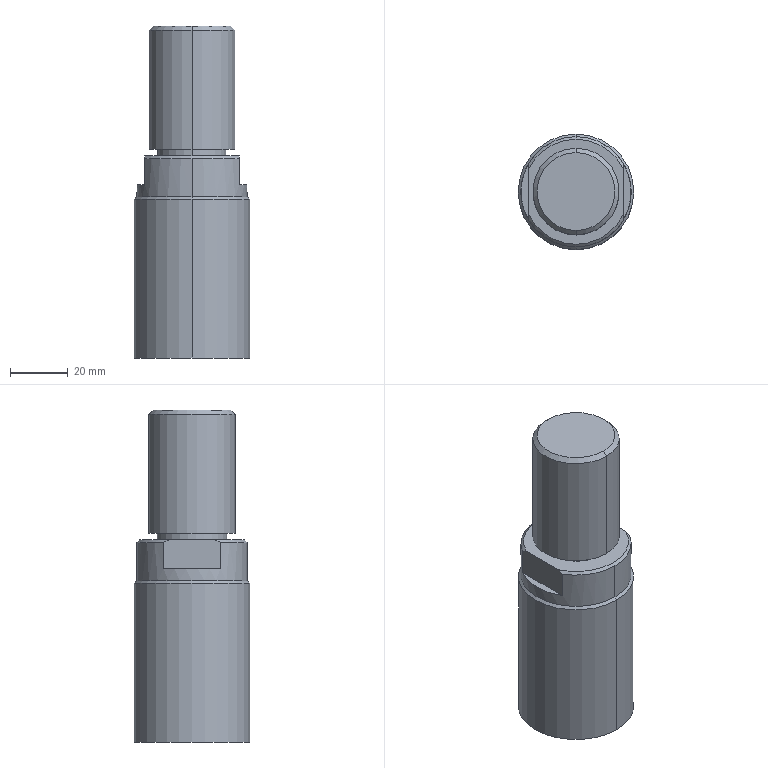Part | SolidWorks | features BaseBody 1 | 1 solid | 23 faces | box 40 x 40 x 115 mm | volume 116741 mm3 | cylinder 8 | plane 8 | cone 7 | commonest cylinder face diameters 24 x2 30 x2 38.2 x2 40 x2
STEP:
#1=CARTESIAN_POINT('',(0.,-13.5,65.));
#2=VERTEX_POINT('',#1);
#3=CARTESIAN_POINT('',(0.,13.5,65.));
#4=VERTEX_POINT('',#3);
#5=CARTESIAN_POINT('',(0.,0.,65.));
#6=DIRECTION('',(0.,0.,1.));
#7=DIRECTION('',(0.,-1.,0.));
#8=AXIS2_PLACEMENT_3D('',#5,#6,#7);
#9=CIRCLE('',#8,13.5);
#10=EDGE_CURVE('',#2,#4,#9,.T.);
#11=ORIENTED_EDGE('',*,*,#10,.F.);
#12=CARTESIAN_POINT('',(0.,-15.,63.5));
#13=VERTEX_POINT('',#12);
#14=CARTESIAN_POINT('',(0.,-15.,63.5));
#15=DIRECTION('',(0.,-0.7071,-0.7071));
#16=VECTOR('',#15,1000.);
#17=LINE('',#14,#16);
#18=EDGE_CURVE('',#2,#13,#17,.T.);
#19=ORIENTED_EDGE('',*,*,#18,.T.);
#20=CARTESIAN_POINT('',(0.,15.,63.5));
#21=VERTEX_POINT('',#20);
#22=CARTESIAN_POINT('',(0.,0.,63.5));
#23=DIRECTION('',(0.,0.,-1.));
#24=DIRECTION('',(0.,-1.,0.));
#25=AXIS2_PLACEMENT_3D('',#22,#23,#24);
#26=CIRCLE('',#25,15.);
#27=EDGE_CURVE('',#21,#13,#26,.T.);
#28=ORIENTED_EDGE('',*,*,#27,.F.);
#29=CARTESIAN_POINT('',(0.,15.,63.5));
#30=DIRECTION('',(0.,0.7071,-0.7071));
#31=VECTOR('',#30,1000.);
#32=LINE('',#29,#31);
#33=EDGE_CURVE('',#4,#21,#32,.T.);
#34=ORIENTED_EDGE('',*,*,#33,.F.);
#35=EDGE_LOOP('',(#11,#19,#28,#34));
#36=FACE_OUTER_BOUND('',#35,.T.);
#37=CARTESIAN_POINT('',(0.,0.,63.5));
#38=DIRECTION('',(0.,0.,-1.));
#39=DIRECTION('',(0.,1.,0.));
#40=AXIS2_PLACEMENT_3D('',#37,#38,#39);
#41=CONICAL_SURFACE('',#40,15.,0.7854);
#42=ADVANCED_FACE('',(#36),#41,.T.);
#43=CARTESIAN_POINT('',(0.,20.,5.));
#44=VERTEX_POINT('',#43);
#45=CARTESIAN_POINT('',(0.,-20.,5.));
#46=VERTEX_POINT('',#45);
#47=CARTESIAN_POINT('',(0.,0.,5.));
#48=DIRECTION('',(0.,0.,-1.));
#49=DIRECTION('',(0.,1.,0.));
#50=AXIS2_PLACEMENT_3D('',#47,#48,#49);
#51=CIRCLE('',#50,20.);
#52=EDGE_CURVE('',#44,#46,#51,.T.);
#53=ORIENTED_EDGE('',*,*,#52,.T.);
#54=CARTESIAN_POINT('',(0.,-20.,-50.));
#55=VERTEX_POINT('',#54);
#56=CARTESIAN_POINT('',(0.,-20.,-50.));
#57=DIRECTION('',(0.,0.,-1.));
#58=VECTOR('',#57,1000.);
#59=LINE('',#56,#58);
#60=EDGE_CURVE('',#46,#55,#59,.T.);
#61=ORIENTED_EDGE('',*,*,#60,.T.);
#62=CARTESIAN_POINT('',(0.,20.,-50.));
#63=VERTEX_POINT('',#62);
#64=CARTESIAN_POINT('',(0.,0.,-50.));
#65=DIRECTION('',(0.,0.,-1.));
#66=DIRECTION('',(0.,1.,0.));
#67=AXIS2_PLACEMENT_3D('',#64,#65,#66);
#68=CIRCLE('',#67,20.);
#69=EDGE_CURVE('',#63,#55,#68,.T.);
#70=ORIENTED_EDGE('',*,*,#69,.F.);
#71=CARTESIAN_POINT('',(0.,20.,-50.));
#72=DIRECTION('',(0.,0.,-1.));
#73=VECTOR('',#72,1000.);
#74=LINE('',#71,#73);
#75=EDGE_CURVE('',#44,#63,#74,.T.);
#76=ORIENTED_EDGE('',*,*,#75,.F.);
#77=EDGE_LOOP('',(#53,#61,#70,#76));
#78=FACE_OUTER_BOUND('',#77,.T.);
#79=CARTESIAN_POINT('',(0.,0.,-50.));
#80=DIRECTION('',(0.,0.,-1.));
#81=DIRECTION('',(0.,1.,0.));
#82=AXIS2_PLACEMENT_3D('',#79,#80,#81);
#83=CYLINDRICAL_SURFACE('',#82,20.);
#84=ADVANCED_FACE('',(#78),#83,.T.);
#85=CARTESIAN_POINT('',(0.,19.1,5.9));
#86=VERTEX_POINT('',#85);
#87=CARTESIAN_POINT('',(0.,-19.1,5.9));
#88=VERTEX_POINT('',#87);
#89=CARTESIAN_POINT('',(0.,0.,5.9));
#90=DIRECTION('',(0.,0.,-1.));
#91=DIRECTION('',(0.,1.,0.));
#92=AXIS2_PLACEMENT_3D('',#89,#90,#91);
#93=CIRCLE('',#92,19.1);
#94=EDGE_CURVE('',#86,#88,#93,.T.);
#95=ORIENTED_EDGE('',*,*,#94,.T.);
#96=CARTESIAN_POINT('',(0.,-20.,5.));
#97=DIRECTION('',(0.,-0.7071,-0.7071));
#98=VECTOR('',#97,1000.);
#99=LINE('',#96,#98);
#100=EDGE_CURVE('',#88,#46,#99,.T.);
#101=ORIENTED_EDGE('',*,*,#100,.T.);
#102=ORIENTED_EDGE('',*,*,#52,.F.);
#103=CARTESIAN_POINT('',(0.,20.,5.));
#104=DIRECTION('',(0.,0.7071,-0.7071));
#105=VECTOR('',#104,1000.);
#106=LINE('',#103,#105);
#107=EDGE_CURVE('',#86,#44,#106,.T.);
#108=ORIENTED_EDGE('',*,*,#107,.F.);
#109=EDGE_LOOP('',(#95,#101,#102,#108));
#110=FACE_OUTER_BOUND('',#109,.T.);
#111=CARTESIAN_POINT('',(0.,0.,5.));
#112=DIRECTION('',(0.,0.,-1.));
#113=DIRECTION('',(0.,1.,0.));
#114=AXIS2_PLACEMENT_3D('',#111,#112,#113);
#115=CONICAL_SURFACE('',#114,20.,0.7854);
#116=ADVANCED_FACE('',(#110),#115,.T.);
#117=CARTESIAN_POINT('',(16.4,-9.79,19.1));
#118=VERTEX_POINT('',#117);
#119=CARTESIAN_POINT('',(0.,-19.1,19.1));
#120=VERTEX_POINT('',#119);
#121=CARTESIAN_POINT('',(0.,0.,19.1));
#122=DIRECTION('',(0.,0.,-1.));
#123=DIRECTION('',(0.,1.,0.));
#124=AXIS2_PLACEMENT_3D('',#121,#122,#123);
#125=CIRCLE('',#124,19.1);
#126=EDGE_CURVE('',#118,#120,#125,.T.);
#127=ORIENTED_EDGE('',*,*,#126,.T.);
#128=CARTESIAN_POINT('',(0.,-19.1,-50.));
#129=DIRECTION('',(0.,0.,-1.));
#130=VECTOR('',#129,1000.);
#131=LINE('',#128,#130);
#132=EDGE_CURVE('',#120,#88,#131,.T.);
#133=ORIENTED_EDGE('',*,*,#132,.T.);
#134=ORIENTED_EDGE('',*,*,#94,.F.);
#135=CARTESIAN_POINT('',(0.,19.1,19.1));
#136=VERTEX_POINT('',#135);
#137=CARTESIAN_POINT('',(0.,19.1,-50.));
#138=DIRECTION('',(0.,0.,-1.));
#139=VECTOR('',#138,1000.);
#140=LINE('',#137,#139);
#141=EDGE_CURVE('',#136,#86,#140,.T.);
#142=ORIENTED_EDGE('',*,*,#141,.F.);
#143=CARTESIAN_POINT('',(16.4,9.79,19.1));
#144=VERTEX_POINT('',#143);
#145=CARTESIAN_POINT('',(0.,0.,19.1));
#146=DIRECTION('',(0.,0.,-1.));
#147=DIRECTION('',(0.,1.,0.));
#148=AXIS2_PLACEMENT_3D('',#145,#146,#147);
#149=CIRCLE('',#148,19.1);
#150=EDGE_CURVE('',#136,#144,#149,.T.);
#151=ORIENTED_EDGE('',*,*,#150,.T.);
#152=CARTESIAN_POINT('',(16.4,9.79,10.));
#153=VERTEX_POINT('',#152);
#154=CARTESIAN_POINT('',(16.4,9.79,10.));
#155=DIRECTION('',(0.,0.,1.));
#156=VECTOR('',#155,1000.);
#157=LINE('',#154,#156);
#158=EDGE_CURVE('',#153,#144,#157,.T.);
#159=ORIENTED_EDGE('',*,*,#158,.F.);
#160=CARTESIAN_POINT('',(16.4,-9.79,10.));
#161=VERTEX_POINT('',#160);
#162=CARTESIAN_POINT('',(0.,0.,10.));
#163=DIRECTION('',(0.,0.,1.));
#164=DIRECTION('',(1.,0.,0.));
#165=AXIS2_PLACEMENT_3D('',#162,#163,#164);
#166=CIRCLE('',#165,19.1);
#167=EDGE_CURVE('',#161,#153,#166,.T.);
#168=ORIENTED_EDGE('',*,*,#167,.F.);
#169=CARTESIAN_POINT('',(16.4,-9.79,10.));
#170=DIRECTION('',(0.,0.,1.));
#171=VECTOR('',#170,1000.);
#172=LINE('',#169,#171);
#173=EDGE_CURVE('',#161,#118,#172,.T.);
#174=ORIENTED_EDGE('',*,*,#173,.T.);
#175=EDGE_LOOP('',(#127,#133,#134,#142,#151,#159,#168,#174));
#176=FACE_OUTER_BOUND('',#175,.T.);
#177=CARTESIAN_POINT('',(0.,0.,-50.));
#178=DIRECTION('',(0.,0.,-1.));
#179=DIRECTION('',(0.,1.,0.));
#180=AXIS2_PLACEMENT_3D('',#177,#178,#179);
#181=CYLINDRICAL_SURFACE('',#180,19.1);
#182=ADVANCED_FACE('',(#176),#181,.T.);
#183=CARTESIAN_POINT('',(0.,12.,22.25));
#184=VERTEX_POINT('',#183);
#185=CARTESIAN_POINT('',(0.,-12.,22.25));
#186=VERTEX_POINT('',#185);
#187=CARTESIAN_POINT('',(0.,0.,22.25));
#188=DIRECTION('',(0.,0.,-1.));
#189=DIRECTION('',(0.,1.,0.));
#190=AXIS2_PLACEMENT_3D('',#187,#188,#189);
#191=CIRCLE('',#190,12.);
#192=EDGE_CURVE('',#184,#186,#191,.T.);
#193=ORIENTED_EDGE('',*,*,#192,.T.);
#194=CARTESIAN_POINT('',(0.,-12.,20.));
#195=VERTEX_POINT('',#194);
#196=CARTESIAN_POINT('',(0.,-12.,-50.));
#197=DIRECTION('',(0.,0.,-1.));
#198=VECTOR('',#197,1000.);
#199=LINE('',#196,#198);
#200=EDGE_CURVE('',#186,#195,#199,.T.);
#201=ORIENTED_EDGE('',*,*,#200,.T.);
#202=CARTESIAN_POINT('',(0.,12.,20.));
#203=VERTEX_POINT('',#202);
#204=CARTESIAN_POINT('',(0.,0.,20.));
#205=DIRECTION('',(0.,0.,-1.));
#206=DIRECTION('',(0.,1.,0.));
#207=AXIS2_PLACEMENT_3D('',#204,#205,#206);
#208=CIRCLE('',#207,12.);
#209=EDGE_CURVE('',#203,#195,#208,.T.);
#210=ORIENTED_EDGE('',*,*,#209,.F.);
#211=CARTESIAN_POINT('',(0.,12.,-50.));
#212=DIRECTION('',(0.,0.,-1.));
#213=VECTOR('',#212,1000.);
#214=LINE('',#211,#213);
#215=EDGE_CURVE('',#184,#203,#214,.T.);
#216=ORIENTED_EDGE('',*,*,#215,.F.);
#217=EDGE_LOOP('',(#193,#201,#210,#216));
#218=FACE_OUTER_BOUND('',#217,.T.);
#219=CARTESIAN_POINT('',(0.,0.,-50.));
#220=DIRECTION('',(0.,0.,-1.));
#221=DIRECTION('',(0.,1.,0.));
#222=AXIS2_PLACEMENT_3D('',#219,#220,#221);
#223=CYLINDRICAL_SURFACE('',#222,12.);
#224=ADVANCED_FACE('',(#218),#223,.T.);
#225=ORIENTED_EDGE('',*,*,#27,.T.);
#226=CARTESIAN_POINT('',(0.,-15.,22.25));
#227=VERTEX_POINT('',#226);
#228=CARTESIAN_POINT('',(0.,-15.,-50.));
#229=DIRECTION('',(0.,0.,-1.));
#230=VECTOR('',#229,1000.);
#231=LINE('',#228,#230);
#232=EDGE_CURVE('',#13,#227,#231,.T.);
#233=ORIENTED_EDGE('',*,*,#232,.T.);
#234=CARTESIAN_POINT('',(0.,15.,22.25));
#235=VERTEX_POINT('',#234);
#236=CARTESIAN_POINT('',(0.,0.,22.25));
#237=DIRECTION('',(0.,0.,-1.));
#238=DIRECTION('',(0.,1.,0.));
#239=AXIS2_PLACEMENT_3D('',#236,#237,#238);
#240=CIRCLE('',#239,15.);
#241=EDGE_CURVE('',#235,#227,#240,.T.);
#242=ORIENTED_EDGE('',*,*,#241,.F.);
#243=CARTESIAN_POINT('',(0.,15.,-50.));
#244=DIRECTION('',(0.,0.,-1.));
#245=VECTOR('',#244,1000.);
#246=LINE('',#243,#245);
#247=EDGE_CURVE('',#21,#235,#246,.T.);
#248=ORIENTED_EDGE('',*,*,#247,.F.);
#249=EDGE_LOOP('',(#225,#233,#242,#248));
#250=FACE_OUTER_BOUND('',#249,.T.);
#251=CARTESIAN_POINT('',(0.,0.,-50.));
#252=DIRECTION('',(0.,0.,-1.));
#253=DIRECTION('',(0.,1.,0.));
#254=AXIS2_PLACEMENT_3D('',#251,#252,#253);
#255=CYLINDRICAL_SURFACE('',#254,15.);
#256=ADVANCED_FACE('',(#250),#255,.T.);
#257=CARTESIAN_POINT('',(-16.4,7.892,20.));
#258=VERTEX_POINT('',#257);
#259=CARTESIAN_POINT('',(0.,18.2,20.));
#260=VERTEX_POINT('',#259);
#261=CARTESIAN_POINT('',(0.,0.,20.));
#262=DIRECTION('',(0.,0.,-1.));
#263=DIRECTION('',(0.,1.,0.));
#264=AXIS2_PLACEMENT_3D('',#261,#262,#263);
#265=CIRCLE('',#264,18.2);
#266=EDGE_CURVE('',#258,#260,#265,.T.);
#267=ORIENTED_EDGE('',*,*,#266,.T.);
#268=CARTESIAN_POINT('',(0.,19.1,19.1));
#269=DIRECTION('',(0.,0.7071,-0.7071));
#270=VECTOR('',#269,1000.);
#271=LINE('',#268,#270);
#272=EDGE_CURVE('',#260,#136,#271,.T.);
#273=ORIENTED_EDGE('',*,*,#272,.T.);
#274=CARTESIAN_POINT('',(-16.4,9.79,19.1));
#275=VERTEX_POINT('',#274);
#276=CARTESIAN_POINT('',(0.,0.,19.1));
#277=DIRECTION('',(0.,0.,-1.));
#278=DIRECTION('',(0.,1.,0.));
#279=AXIS2_PLACEMENT_3D('',#276,#277,#278);
#280=CIRCLE('',#279,19.1);
#281=EDGE_CURVE('',#275,#136,#280,.T.);
#282=ORIENTED_EDGE('',*,*,#281,.F.);
#283=CARTESIAN_POINT('',(-16.4,7.892,20.));
#284=CARTESIAN_POINT('',(-16.4,8.532,19.722));
#285=CARTESIAN_POINT('',(-16.4,9.165,19.42));
#286=CARTESIAN_POINT('',(-16.4,9.79,19.1));
#287=B_SPLINE_CURVE_WITH_KNOTS('',3,(#283,#284,#285,#286),.UNSPECIFIED.,.F.,.F.,(4,4),(0.03257,0.03466),.UNSPECIFIED.);
#288=EDGE_CURVE('',#258,#275,#287,.T.);
#289=ORIENTED_EDGE('',*,*,#288,.F.);
#290=EDGE_LOOP('',(#267,#273,#282,#289));
#291=FACE_OUTER_BOUND('',#290,.T.);
#292=CARTESIAN_POINT('',(0.,0.,19.1));
#293=DIRECTION('',(0.,0.,-1.));
#294=DIRECTION('',(0.,1.,0.));
#295=AXIS2_PLACEMENT_3D('',#292,#293,#294);
#296=CONICAL_SURFACE('',#295,19.1,0.7854);
#297=ADVANCED_FACE('',(#291),#296,.T.);
#298=ORIENTED_EDGE('',*,*,#272,.F.);
#299=CARTESIAN_POINT('',(16.4,7.892,20.));
#300=VERTEX_POINT('',#299);
#301=CARTESIAN_POINT('',(0.,0.,20.));
#302=DIRECTION('',(0.,0.,-1.));
#303=DIRECTION('',(0.,1.,0.));
#304=AXIS2_PLACEMENT_3D('',#301,#302,#303);
#305=CIRCLE('',#304,18.2);
#306=EDGE_CURVE('',#260,#300,#305,.T.);
#307=ORIENTED_EDGE('',*,*,#306,.T.);
#308=CARTESIAN_POINT('',(16.4,9.79,19.1));
#309=CARTESIAN_POINT('',(16.4,9.166,19.42));
#310=CARTESIAN_POINT('',(16.4,8.533,19.722));
#311=CARTESIAN_POINT('',(16.4,7.892,20.));
#312=B_SPLINE_CURVE_WITH_KNOTS('',3,(#308,#309,#310,#311),.UNSPECIFIED.,.F.,.F.,(4,4),(0.01421,0.0163),.UNSPECIFIED.);
#313=EDGE_CURVE('',#144,#300,#312,.T.);
#314=ORIENTED_EDGE('',*,*,#313,.F.);
#315=ORIENTED_EDGE('',*,*,#150,.F.);
#316=EDGE_LOOP('',(#298,#307,#314,#315));
#317=FACE_OUTER_BOUND('',#316,.T.);
#318=CARTESIAN_POINT('',(0.,0.,19.1));
#319=DIRECTION('',(0.,0.,-1.));
#320=DIRECTION('',(0.,1.,0.));
#321=AXIS2_PLACEMENT_3D('',#318,#319,#320);
#322=CONICAL_SURFACE('',#321,19.1,0.7854);
#323=ADVANCED_FACE('',(#317),#322,.T.);
#324=CARTESIAN_POINT('',(0.,0.,65.));
#325=DIRECTION('',(0.,0.,1.));
#326=DIRECTION('',(0.,-1.,0.));
#327=AXIS2_PLACEMENT_3D('',#324,#325,#326);
#328=CIRCLE('',#327,13.5);
#329=EDGE_CURVE('',#4,#2,#328,.T.);
#330=ORIENTED_EDGE('',*,*,#329,.T.);
#331=ORIENTED_EDGE('',*,*,#10,.T.);
#332=EDGE_LOOP('',(#330,#331));
#333=FACE_OUTER_BOUND('',#332,.T.);
#334=CARTESIAN_POINT('',(0.,0.,65.));
#335=DIRECTION('',(0.,0.,1.));
#336=DIRECTION('',(0.,-1.,0.));
#337=AXIS2_PLACEMENT_3D('',#334,#335,#336);
#338=PLANE('',#337);
#339=ADVANCED_FACE('',(#333),#338,.T.);
#340=ORIENTED_EDGE('',*,*,#232,.F.);
#341=CARTESIAN_POINT('',(0.,0.,63.5));
#342=DIRECTION('',(0.,0.,-1.));
#343=DIRECTION('',(0.,-1.,0.));
#344=AXIS2_PLACEMENT_3D('',#341,#342,#343);
#345=CIRCLE('',#344,15.);
#346=EDGE_CURVE('',#13,#21,#345,.T.);
#347=ORIENTED_EDGE('',*,*,#346,.T.);
#348=ORIENTED_EDGE('',*,*,#247,.T.);
#349=CARTESIAN_POINT('',(0.,0.,22.25));
#350=DIRECTION('',(0.,0.,-1.));
#351=DIRECTION('',(0.,1.,0.));
#352=AXIS2_PLACEMENT_3D('',#349,#350,#351);
#353=CIRCLE('',#352,15.);
#354=EDGE_CURVE('',#227,#235,#353,.T.);
#355=ORIENTED_EDGE('',*,*,#354,.F.);
#356=EDGE_LOOP('',(#340,#347,#348,#355));
#357=FACE_OUTER_BOUND('',#356,.T.);
#358=CARTESIAN_POINT('',(0.,0.,-50.));
#359=DIRECTION('',(0.,0.,-1.));
#360=DIRECTION('',(0.,1.,0.));
#361=AXIS2_PLACEMENT_3D('',#358,#359,#360);
#362=CYLINDRICAL_SURFACE('',#361,15.);
#363=ADVANCED_FACE('',(#357),#362,.T.);
#364=ORIENTED_EDGE('',*,*,#241,.T.);
#365=ORIENTED_EDGE('',*,*,#354,.T.);
#366=EDGE_LOOP('',(#364,#365));
#367=FACE_OUTER_BOUND('',#366,.T.);
#368=ORIENTED_EDGE('',*,*,#192,.F.);
#369=CARTESIAN_POINT('',(0.,0.,22.25));
#370=DIRECTION('',(0.,0.,-1.));
#371=DIRECTION('',(0.,1.,0.));
#372=AXIS2_PLACEMENT_3D('',#369,#370,#371);
#373=CIRCLE('',#372,12.);
#374=EDGE_CURVE('',#186,#184,#373,.T.);
#375=ORIENTED_EDGE('',*,*,#374,.F.);
#376=EDGE_LOOP('',(#368,#375));
#377=FACE_BOUND('',#376,.T.);
#378=CARTESIAN_POINT('',(0.,-15.,22.25));
#379=DIRECTION('',(0.,0.,-1.));
#380=DIRECTION('',(0.,1.,0.));
#381=AXIS2_PLACEMENT_3D('',#378,#379,#380);
#382=PLANE('',#381);
#383=ADVANCED_FACE('',(#367,#377),#382,.T.);
#384=ORIENTED_EDGE('',*,*,#200,.F.);
#385=ORIENTED_EDGE('',*,*,#374,.T.);
#386=ORIENTED_EDGE('',*,*,#215,.T.);
#387=CARTESIAN_POINT('',(0.,0.,20.));
#388=DIRECTION('',(0.,0.,-1.));
#389=DIRECTION('',(0.,1.,0.));
#390=AXIS2_PLACEMENT_3D('',#387,#388,#389);
#391=CIRCLE('',#390,12.);
#392=EDGE_CURVE('',#195,#203,#391,.T.);
#393=ORIENTED_EDGE('',*,*,#392,.F.);
#394=EDGE_LOOP('',(#384,#385,#386,#393));
#395=FACE_OUTER_BOUND('',#394,.T.);
#396=CARTESIAN_POINT('',(0.,0.,-50.));
#397=DIRECTION('',(0.,0.,-1.));
#398=DIRECTION('',(0.,1.,0.));
#399=AXIS2_PLACEMENT_3D('',#396,#397,#398);
#400=CYLINDRICAL_SURFACE('',#399,12.);
#401=ADVANCED_FACE('',(#395),#400,.T.);
#402=CARTESIAN_POINT('',(16.4,-7.892,20.));
#403=VERTEX_POINT('',#402);
#404=CARTESIAN_POINT('',(16.4,9.79,20.));
#405=DIRECTION('',(0.,-1.,0.));
#406=VECTOR('',#405,1000.);
#407=LINE('',#404,#406);
#408=EDGE_CURVE('',#300,#403,#407,.T.);
#409=ORIENTED_EDGE('',*,*,#408,.F.);
#410=ORIENTED_EDGE('',*,*,#306,.F.);
#411=ORIENTED_EDGE('',*,*,#266,.F.);
#412=CARTESIAN_POINT('',(-16.4,-7.892,20.));
#413=VERTEX_POINT('',#412);
#414=CARTESIAN_POINT('',(-16.4,9.79,20.));
#415=DIRECTION('',(0.,1.,0.));
#416=VECTOR('',#415,1000.);
#417=LINE('',#414,#416);
#418=EDGE_CURVE('',#413,#258,#417,.T.);
#419=ORIENTED_EDGE('',*,*,#418,.F.);
#420=CARTESIAN_POINT('',(0.,0.,20.));
#421=DIRECTION('',(0.,0.,-1.));
#422=DIRECTION('',(0.,1.,0.));
#423=AXIS2_PLACEMENT_3D('',#420,#421,#422);
#424=CIRCLE('',#423,18.2);
#425=EDGE_CURVE('',#403,#413,#424,.T.);
#426=ORIENTED_EDGE('',*,*,#425,.F.);
#427=EDGE_LOOP('',(#409,#410,#411,#419,#426));
#428=FACE_OUTER_BOUND('',#427,.T.);
#429=ORIENTED_EDGE('',*,*,#209,.T.);
#430=ORIENTED_EDGE('',*,*,#392,.T.);
#431=EDGE_LOOP('',(#429,#430));
#432=FACE_BOUND('',#431,.T.);
#433=CARTESIAN_POINT('',(0.,-12.,20.));
#434=DIRECTION('',(0.,0.,1.));
#435=DIRECTION('',(0.,-1.,0.));
#436=AXIS2_PLACEMENT_3D('',#433,#434,#435);
#437=PLANE('',#436);
#438=ADVANCED_FACE('',(#428,#432),#437,.T.);
#439=CARTESIAN_POINT('',(16.4,-7.892,20.));
#440=CARTESIAN_POINT('',(16.4,-8.532,19.722));
#441=CARTESIAN_POINT('',(16.4,-9.165,19.42));
#442=CARTESIAN_POINT('',(16.4,-9.79,19.1));
#443=B_SPLINE_CURVE_WITH_KNOTS('',3,(#439,#440,#441,#442),.UNSPECIFIED.,.F.,.F.,(4,4),(0.03257,0.03466),.UNSPECIFIED.);
#444=EDGE_CURVE('',#403,#118,#443,.T.);
#445=ORIENTED_EDGE('',*,*,#444,.F.);
#446=ORIENTED_EDGE('',*,*,#425,.T.);
#447=CARTESIAN_POINT('',(-16.4,-9.79,19.1));
#448=VERTEX_POINT('',#447);
#449=CARTESIAN_POINT('',(-16.4,-9.79,19.1));
#450=CARTESIAN_POINT('',(-16.4,-9.166,19.42));
#451=CARTESIAN_POINT('',(-16.4,-8.533,19.722));
#452=CARTESIAN_POINT('',(-16.4,-7.892,20.));
#453=B_SPLINE_CURVE_WITH_KNOTS('',3,(#449,#450,#451,#452),.UNSPECIFIED.,.F.,.F.,(4,4),(0.01421,0.0163),.UNSPECIFIED.);
#454=EDGE_CURVE('',#448,#413,#453,.T.);
#455=ORIENTED_EDGE('',*,*,#454,.F.);
#456=CARTESIAN_POINT('',(0.,0.,19.1));
#457=DIRECTION('',(0.,0.,-1.));
#458=DIRECTION('',(0.,1.,0.));
#459=AXIS2_PLACEMENT_3D('',#456,#457,#458);
#460=CIRCLE('',#459,19.1);
#461=EDGE_CURVE('',#120,#448,#460,.T.);
#462=ORIENTED_EDGE('',*,*,#461,.F.);
#463=ORIENTED_EDGE('',*,*,#126,.F.);
#464=EDGE_LOOP('',(#445,#446,#455,#462,#463));
#465=FACE_OUTER_BOUND('',#464,.T.);
#466=CARTESIAN_POINT('',(0.,0.,19.1));
#467=DIRECTION('',(0.,0.,-1.));
#468=DIRECTION('',(0.,1.,0.));
#469=AXIS2_PLACEMENT_3D('',#466,#467,#468);
#470=CONICAL_SURFACE('',#469,19.1,0.7854);
#471=ADVANCED_FACE('',(#465),#470,.T.);
#472=ORIENTED_EDGE('',*,*,#132,.F.);
#473=ORIENTED_EDGE('',*,*,#461,.T.);
#474=CARTESIAN_POINT('',(-16.4,-9.79,10.));
#475=VERTEX_POINT('',#474);
#476=CARTESIAN_POINT('',(-16.4,-9.79,10.));
#477=DIRECTION('',(0.,0.,1.));
#478=VECTOR('',#477,1000.);
#479=LINE('',#476,#478);
#480=EDGE_CURVE('',#475,#448,#479,.T.);
#481=ORIENTED_EDGE('',*,*,#480,.F.);
#482=CARTESIAN_POINT('',(-16.4,9.79,10.));
#483=VERTEX_POINT('',#482);
#484=CARTESIAN_POINT('',(0.,0.,10.));
#485=DIRECTION('',(0.,0.,1.));
#486=DIRECTION('',(1.,0.,0.));
#487=AXIS2_PLACEMENT_3D('',#484,#485,#486);
#488=CIRCLE('',#487,19.1);
#489=EDGE_CURVE('',#483,#475,#488,.T.);
#490=ORIENTED_EDGE('',*,*,#489,.F.);
#491=CARTESIAN_POINT('',(-16.4,9.79,10.));
#492=DIRECTION('',(0.,0.,1.));
#493=VECTOR('',#492,1000.);
#494=LINE('',#491,#493);
#495=EDGE_CURVE('',#483,#275,#494,.T.);
#496=ORIENTED_EDGE('',*,*,#495,.T.);
#497=ORIENTED_EDGE('',*,*,#281,.T.);
#498=ORIENTED_EDGE('',*,*,#141,.T.);
#499=CARTESIAN_POINT('',(0.,0.,5.9));
#500=DIRECTION('',(0.,0.,-1.));
#501=DIRECTION('',(0.,1.,0.));
#502=AXIS2_PLACEMENT_3D('',#499,#500,#501);
#503=CIRCLE('',#502,19.1);
#504=EDGE_CURVE('',#88,#86,#503,.T.);
#505=ORIENTED_EDGE('',*,*,#504,.F.);
#506=EDGE_LOOP('',(#472,#473,#481,#490,#496,#497,#498,#505));
#507=FACE_OUTER_BOUND('',#506,.T.);
#508=CARTESIAN_POINT('',(0.,0.,-50.));
#509=DIRECTION('',(0.,0.,-1.));
#510=DIRECTION('',(0.,1.,0.));
#511=AXIS2_PLACEMENT_3D('',#508,#509,#510);
#512=CYLINDRICAL_SURFACE('',#511,19.1);
#513=ADVANCED_FACE('',(#507),#512,.T.);
#514=ORIENTED_EDGE('',*,*,#100,.F.);
#515=ORIENTED_EDGE('',*,*,#504,.T.);
#516=ORIENTED_EDGE('',*,*,#107,.T.);
#517=CARTESIAN_POINT('',(0.,0.,5.));
#518=DIRECTION('',(0.,0.,-1.));
#519=DIRECTION('',(0.,1.,0.));
#520=AXIS2_PLACEMENT_3D('',#517,#518,#519);
#521=CIRCLE('',#520,20.);
#522=EDGE_CURVE('',#46,#44,#521,.T.);
#523=ORIENTED_EDGE('',*,*,#522,.F.);
#524=EDGE_LOOP('',(#514,#515,#516,#523));
#525=FACE_OUTER_BOUND('',#524,.T.);
#526=CARTESIAN_POINT('',(0.,0.,5.));
#527=DIRECTION('',(0.,0.,-1.));
#528=DIRECTION('',(0.,1.,0.));
#529=AXIS2_PLACEMENT_3D('',#526,#527,#528);
#530=CONICAL_SURFACE('',#529,20.,0.7854);
#531=ADVANCED_FACE('',(#525),#530,.T.);
#532=ORIENTED_EDGE('',*,*,#60,.F.);
#533=ORIENTED_EDGE('',*,*,#522,.T.);
#534=ORIENTED_EDGE('',*,*,#75,.T.);
#535=CARTESIAN_POINT('',(0.,0.,-50.));
#536=DIRECTION('',(0.,0.,-1.));
#537=DIRECTION('',(0.,1.,0.));
#538=AXIS2_PLACEMENT_3D('',#535,#536,#537);
#539=CIRCLE('',#538,20.);
#540=EDGE_CURVE('',#55,#63,#539,.T.);
#541=ORIENTED_EDGE('',*,*,#540,.F.);
#542=EDGE_LOOP('',(#532,#533,#534,#541));
#543=FACE_OUTER_BOUND('',#542,.T.);
#544=CARTESIAN_POINT('',(0.,0.,-50.));
#545=DIRECTION('',(0.,0.,-1.));
#546=DIRECTION('',(0.,1.,0.));
#547=AXIS2_PLACEMENT_3D('',#544,#545,#546);
#548=CYLINDRICAL_SURFACE('',#547,20.);
#549=ADVANCED_FACE('',(#543),#548,.T.);
#550=ORIENTED_EDGE('',*,*,#69,.T.);
#551=ORIENTED_EDGE('',*,*,#540,.T.);
#552=EDGE_LOOP('',(#550,#551));
#553=FACE_OUTER_BOUND('',#552,.T.);
#554=CARTESIAN_POINT('',(0.,-20.,-50.));
#555=DIRECTION('',(0.,0.,-1.));
#556=DIRECTION('',(0.,1.,0.));
#557=AXIS2_PLACEMENT_3D('',#554,#555,#556);
#558=PLANE('',#557);
#559=ADVANCED_FACE('',(#553),#558,.T.);
#560=ORIENTED_EDGE('',*,*,#454,.T.);
#561=ORIENTED_EDGE('',*,*,#418,.T.);
#562=ORIENTED_EDGE('',*,*,#288,.T.);
#563=ORIENTED_EDGE('',*,*,#495,.F.);
#564=CARTESIAN_POINT('',(-16.4,9.79,10.));
#565=DIRECTION('',(0.,1.,0.));
#566=VECTOR('',#565,1000.);
#567=LINE('',#564,#566);
#568=EDGE_CURVE('',#475,#483,#567,.T.);
#569=ORIENTED_EDGE('',*,*,#568,.F.);
#570=ORIENTED_EDGE('',*,*,#480,.T.);
#571=EDGE_LOOP('',(#560,#561,#562,#563,#569,#570));
#572=FACE_OUTER_BOUND('',#571,.T.);
#573=CARTESIAN_POINT('',(-16.4,9.79,10.));
#574=DIRECTION('',(1.,0.,0.));
#575=DIRECTION('',(0.,1.,0.));
#576=AXIS2_PLACEMENT_3D('',#573,#574,#575);
#577=PLANE('',#576);
#578=ADVANCED_FACE('',(#572),#577,.F.);
#579=ORIENTED_EDGE('',*,*,#489,.T.);
#580=ORIENTED_EDGE('',*,*,#568,.T.);
#581=EDGE_LOOP('',(#579,#580));
#582=FACE_OUTER_BOUND('',#581,.T.);
#583=CARTESIAN_POINT('',(0.,0.,10.));
#584=DIRECTION('',(0.,0.,1.));
#585=DIRECTION('',(1.,0.,0.));
#586=AXIS2_PLACEMENT_3D('',#583,#584,#585);
#587=PLANE('',#586);
#588=ADVANCED_FACE('',(#582),#587,.T.);
#589=ORIENTED_EDGE('',*,*,#313,.T.);
#590=ORIENTED_EDGE('',*,*,#408,.T.);
#591=ORIENTED_EDGE('',*,*,#444,.T.);
#592=ORIENTED_EDGE('',*,*,#173,.F.);
#593=CARTESIAN_POINT('',(16.4,9.79,10.));
#594=DIRECTION('',(0.,-1.,0.));
#595=VECTOR('',#594,1000.);
#596=LINE('',#593,#595);
#597=EDGE_CURVE('',#153,#161,#596,.T.);
#598=ORIENTED_EDGE('',*,*,#597,.F.);
#599=ORIENTED_EDGE('',*,*,#158,.T.);
#600=EDGE_LOOP('',(#589,#590,#591,#592,#598,#599));
#601=FACE_OUTER_BOUND('',#600,.T.);
#602=CARTESIAN_POINT('',(16.4,9.79,10.));
#603=DIRECTION('',(-1.,0.,0.));
#604=DIRECTION('',(0.,-1.,0.));
#605=AXIS2_PLACEMENT_3D('',#602,#603,#604);
#606=PLANE('',#605);
#607=ADVANCED_FACE('',(#601),#606,.F.);
#608=ORIENTED_EDGE('',*,*,#167,.T.);
#609=ORIENTED_EDGE('',*,*,#597,.T.);
#610=EDGE_LOOP('',(#608,#609));
#611=FACE_OUTER_BOUND('',#610,.T.);
#612=CARTESIAN_POINT('',(0.,0.,10.));
#613=DIRECTION('',(0.,0.,1.));
#614=DIRECTION('',(1.,0.,0.));
#615=AXIS2_PLACEMENT_3D('',#612,#613,#614);
#616=PLANE('',#615);
#617=ADVANCED_FACE('',(#611),#616,.T.);
#618=ORIENTED_EDGE('',*,*,#18,.F.);
#619=ORIENTED_EDGE('',*,*,#329,.F.);
#620=ORIENTED_EDGE('',*,*,#33,.T.);
#621=ORIENTED_EDGE('',*,*,#346,.F.);
#622=EDGE_LOOP('',(#618,#619,#620,#621));
#623=FACE_OUTER_BOUND('',#622,.T.);
#624=CARTESIAN_POINT('',(0.,0.,63.5));
#625=DIRECTION('',(0.,0.,-1.));
#626=DIRECTION('',(0.,1.,0.));
#627=AXIS2_PLACEMENT_3D('',#624,#625,#626);
#628=CONICAL_SURFACE('',#627,15.,0.7854);
#629=ADVANCED_FACE('',(#623),#628,.T.);
#630=CLOSED_SHELL('',(#42,#84,#116,#182,#224,#256,#297,#323,#339,#363,#383,#401,#438,#471,#513,#531,#549,#559,#578,#588,#607,#617,#629));
#631=MANIFOLD_SOLID_BREP('',#630);
#632=CARTESIAN_POINT('',(0.,0.,0.));
#633=DIRECTION('',(0.,0.,1.));
#634=DIRECTION('',(1.,0.,0.));
#635=AXIS2_PLACEMENT_3D('',#632,#633,#634);
#636=(LENGTH_UNIT()NAMED_UNIT(*)SI_UNIT(.MILLI.,.METRE.));
#637=UNCERTAINTY_MEASURE_WITH_UNIT(LENGTH_MEASURE(0.00001),#636,'','');
#638=(NAMED_UNIT(*)PLANE_ANGLE_UNIT()SI_UNIT($,.RADIAN.));
#639=(NAMED_UNIT(*)SI_UNIT($,.STERADIAN.)SOLID_ANGLE_UNIT());
#640=(GEOMETRIC_REPRESENTATION_CONTEXT(3)GLOBAL_UNCERTAINTY_ASSIGNED_CONTEXT((#637))GLOBAL_UNIT_ASSIGNED_CONTEXT((#636,#638,#639))REPRESENTATION_CONTEXT('',''));
#641=ADVANCED_BREP_SHAPE_REPRESENTATION('',(#631,#635),#640);